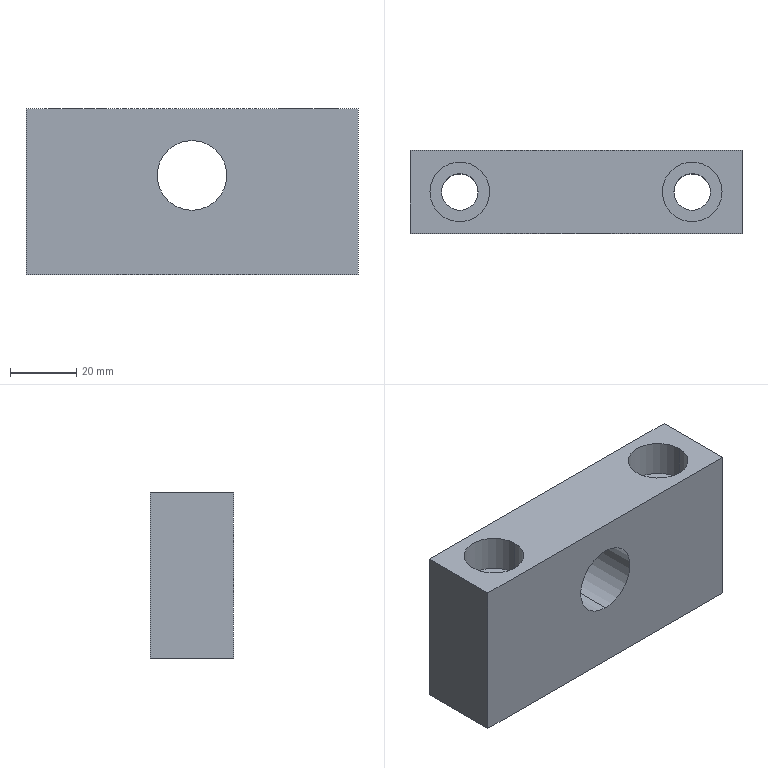Part | SolidWorks | features BaseBody 1 | 1 solid | 26 faces | box 100 x 25 x 50 mm | volume 100070 mm3 | cylinder 14 | plane 8 | cone 4 | commonest cylinder face diameters 10 x4 11 x4 18 x4 21 x2
STEP:
#1=CARTESIAN_POINT('',(20.,0.,19.75));
#2=VERTEX_POINT('',#1);
#3=CARTESIAN_POINT('',(10.,0.,19.75));
#4=VERTEX_POINT('',#3);
#5=CARTESIAN_POINT('',(15.,0.,19.75));
#6=DIRECTION('',(0.,0.,-1.));
#7=DIRECTION('',(-1.,0.,0.));
#8=AXIS2_PLACEMENT_3D('',#5,#6,#7);
#9=CIRCLE('',#8,5.);
#10=EDGE_CURVE('',#2,#4,#9,.T.);
#11=ORIENTED_EDGE('',*,*,#10,.F.);
#12=CARTESIAN_POINT('',(20.,0.,0.));
#13=VERTEX_POINT('',#12);
#14=CARTESIAN_POINT('',(20.,0.,0.));
#15=DIRECTION('',(0.,0.,-1.));
#16=VECTOR('',#15,1000.);
#17=LINE('',#14,#16);
#18=EDGE_CURVE('',#2,#13,#17,.T.);
#19=ORIENTED_EDGE('',*,*,#18,.T.);
#20=CARTESIAN_POINT('',(10.,0.,0.));
#21=VERTEX_POINT('',#20);
#22=CARTESIAN_POINT('',(15.,0.,0.));
#23=DIRECTION('',(0.,0.,-1.));
#24=DIRECTION('',(-1.,0.,0.));
#25=AXIS2_PLACEMENT_3D('',#22,#23,#24);
#26=CIRCLE('',#25,5.);
#27=EDGE_CURVE('',#13,#21,#26,.T.);
#28=ORIENTED_EDGE('',*,*,#27,.T.);
#29=CARTESIAN_POINT('',(10.,0.,0.));
#30=DIRECTION('',(0.,0.,-1.));
#31=VECTOR('',#30,1000.);
#32=LINE('',#29,#31);
#33=EDGE_CURVE('',#4,#21,#32,.T.);
#34=ORIENTED_EDGE('',*,*,#33,.F.);
#35=EDGE_LOOP('',(#11,#19,#28,#34));
#36=FACE_OUTER_BOUND('',#35,.T.);
#37=CARTESIAN_POINT('',(15.,0.,0.));
#38=DIRECTION('',(0.,0.,-1.));
#39=DIRECTION('',(-1.,0.,0.));
#40=AXIS2_PLACEMENT_3D('',#37,#38,#39);
#41=CYLINDRICAL_SURFACE('',#40,5.);
#42=ADVANCED_FACE('',(#36),#41,.F.);
#43=CARTESIAN_POINT('',(15.,0.,22.754));
#44=VERTEX_POINT('',#43);
#45=CARTESIAN_POINT('',(10.,0.,19.75));
#46=DIRECTION('',(-0.8572,0.,-0.515));
#47=VECTOR('',#46,1000.);
#48=LINE('',#45,#47);
#49=EDGE_CURVE('',#44,#4,#48,.T.);
#50=ORIENTED_EDGE('',*,*,#49,.F.);
#51=CARTESIAN_POINT('',(20.,0.,19.75));
#52=DIRECTION('',(0.8572,0.,-0.515));
#53=VECTOR('',#52,1000.);
#54=LINE('',#51,#53);
#55=EDGE_CURVE('',#44,#2,#54,.T.);
#56=ORIENTED_EDGE('',*,*,#55,.T.);
#57=ORIENTED_EDGE('',*,*,#10,.T.);
#58=EDGE_LOOP('',(#50,#56,#57));
#59=FACE_OUTER_BOUND('',#58,.T.);
#60=CARTESIAN_POINT('',(15.,0.,19.75));
#61=DIRECTION('',(0.,0.,-1.));
#62=DIRECTION('',(-1.,0.,0.));
#63=AXIS2_PLACEMENT_3D('',#60,#61,#62);
#64=CONICAL_SURFACE('',#63,5.,1.03);
#65=ADVANCED_FACE('',(#59),#64,.F.);
#66=CARTESIAN_POINT('',(-10.,0.,19.75));
#67=VERTEX_POINT('',#66);
#68=CARTESIAN_POINT('',(-20.,0.,19.75));
#69=VERTEX_POINT('',#68);
#70=CARTESIAN_POINT('',(-15.,0.,19.75));
#71=DIRECTION('',(0.,0.,-1.));
#72=DIRECTION('',(-1.,0.,0.));
#73=AXIS2_PLACEMENT_3D('',#70,#71,#72);
#74=CIRCLE('',#73,5.);
#75=EDGE_CURVE('',#67,#69,#74,.T.);
#76=ORIENTED_EDGE('',*,*,#75,.F.);
#77=CARTESIAN_POINT('',(-10.,0.,0.));
#78=VERTEX_POINT('',#77);
#79=CARTESIAN_POINT('',(-10.,0.,0.));
#80=DIRECTION('',(0.,0.,-1.));
#81=VECTOR('',#80,1000.);
#82=LINE('',#79,#81);
#83=EDGE_CURVE('',#67,#78,#82,.T.);
#84=ORIENTED_EDGE('',*,*,#83,.T.);
#85=CARTESIAN_POINT('',(-20.,0.,0.));
#86=VERTEX_POINT('',#85);
#87=CARTESIAN_POINT('',(-15.,0.,0.));
#88=DIRECTION('',(0.,0.,-1.));
#89=DIRECTION('',(-1.,0.,0.));
#90=AXIS2_PLACEMENT_3D('',#87,#88,#89);
#91=CIRCLE('',#90,5.);
#92=EDGE_CURVE('',#78,#86,#91,.T.);
#93=ORIENTED_EDGE('',*,*,#92,.T.);
#94=CARTESIAN_POINT('',(-20.,0.,0.));
#95=DIRECTION('',(0.,0.,-1.));
#96=VECTOR('',#95,1000.);
#97=LINE('',#94,#96);
#98=EDGE_CURVE('',#69,#86,#97,.T.);
#99=ORIENTED_EDGE('',*,*,#98,.F.);
#100=EDGE_LOOP('',(#76,#84,#93,#99));
#101=FACE_OUTER_BOUND('',#100,.T.);
#102=CARTESIAN_POINT('',(-15.,0.,0.));
#103=DIRECTION('',(0.,0.,-1.));
#104=DIRECTION('',(-1.,0.,0.));
#105=AXIS2_PLACEMENT_3D('',#102,#103,#104);
#106=CYLINDRICAL_SURFACE('',#105,5.);
#107=ADVANCED_FACE('',(#101),#106,.F.);
#108=CARTESIAN_POINT('',(-15.,0.,22.754));
#109=VERTEX_POINT('',#108);
#110=CARTESIAN_POINT('',(-20.,0.,19.75));
#111=DIRECTION('',(-0.8572,0.,-0.515));
#112=VECTOR('',#111,1000.);
#113=LINE('',#110,#112);
#114=EDGE_CURVE('',#109,#69,#113,.T.);
#115=ORIENTED_EDGE('',*,*,#114,.F.);
#116=CARTESIAN_POINT('',(-10.,0.,19.75));
#117=DIRECTION('',(0.8572,0.,-0.515));
#118=VECTOR('',#117,1000.);
#119=LINE('',#116,#118);
#120=EDGE_CURVE('',#109,#67,#119,.T.);
#121=ORIENTED_EDGE('',*,*,#120,.T.);
#122=ORIENTED_EDGE('',*,*,#75,.T.);
#123=EDGE_LOOP('',(#115,#121,#122));
#124=FACE_OUTER_BOUND('',#123,.T.);
#125=CARTESIAN_POINT('',(-15.,0.,19.75));
#126=DIRECTION('',(0.,0.,-1.));
#127=DIRECTION('',(-1.,0.,0.));
#128=AXIS2_PLACEMENT_3D('',#125,#126,#127);
#129=CONICAL_SURFACE('',#128,5.,1.03);
#130=ADVANCED_FACE('',(#124),#129,.F.);
#131=CARTESIAN_POINT('',(0.,-12.5,19.5));
#132=VERTEX_POINT('',#131);
#133=CARTESIAN_POINT('',(0.,-12.5,40.5));
#134=VERTEX_POINT('',#133);
#135=CARTESIAN_POINT('',(0.,-12.5,30.));
#136=DIRECTION('',(0.,1.,0.));
#137=DIRECTION('',(0.,0.,1.));
#138=AXIS2_PLACEMENT_3D('',#135,#136,#137);
#139=CIRCLE('',#138,10.5);
#140=EDGE_CURVE('',#132,#134,#139,.T.);
#141=ORIENTED_EDGE('',*,*,#140,.F.);
#142=CARTESIAN_POINT('',(0.,12.5,19.5));
#143=VERTEX_POINT('',#142);
#144=CARTESIAN_POINT('',(0.,12.5,19.5));
#145=DIRECTION('',(0.,1.,0.));
#146=VECTOR('',#145,1000.);
#147=LINE('',#144,#146);
#148=EDGE_CURVE('',#132,#143,#147,.T.);
#149=ORIENTED_EDGE('',*,*,#148,.T.);
#150=CARTESIAN_POINT('',(0.,12.5,40.5));
#151=VERTEX_POINT('',#150);
#152=CARTESIAN_POINT('',(0.,12.5,30.));
#153=DIRECTION('',(0.,1.,0.));
#154=DIRECTION('',(0.,0.,1.));
#155=AXIS2_PLACEMENT_3D('',#152,#153,#154);
#156=CIRCLE('',#155,10.5);
#157=EDGE_CURVE('',#143,#151,#156,.T.);
#158=ORIENTED_EDGE('',*,*,#157,.T.);
#159=CARTESIAN_POINT('',(0.,12.5,40.5));
#160=DIRECTION('',(0.,1.,0.));
#161=VECTOR('',#160,1000.);
#162=LINE('',#159,#161);
#163=EDGE_CURVE('',#134,#151,#162,.T.);
#164=ORIENTED_EDGE('',*,*,#163,.F.);
#165=EDGE_LOOP('',(#141,#149,#158,#164));
#166=FACE_OUTER_BOUND('',#165,.T.);
#167=CARTESIAN_POINT('',(0.,12.5,30.));
#168=DIRECTION('',(0.,1.,0.));
#169=DIRECTION('',(0.,0.,1.));
#170=AXIS2_PLACEMENT_3D('',#167,#168,#169);
#171=CYLINDRICAL_SURFACE('',#170,10.5);
#172=ADVANCED_FACE('',(#166),#171,.F.);
#173=CARTESIAN_POINT('',(-44.,0.,39.));
#174=VERTEX_POINT('',#173);
#175=CARTESIAN_POINT('',(-26.,0.,39.));
#176=VERTEX_POINT('',#175);
#177=CARTESIAN_POINT('',(-35.,0.,39.));
#178=DIRECTION('',(0.,0.,1.));
#179=DIRECTION('',(1.,0.,0.));
#180=AXIS2_PLACEMENT_3D('',#177,#178,#179);
#181=CIRCLE('',#180,9.);
#182=EDGE_CURVE('',#174,#176,#181,.T.);
#183=ORIENTED_EDGE('',*,*,#182,.F.);
#184=CARTESIAN_POINT('',(-44.,0.,50.));
#185=VERTEX_POINT('',#184);
#186=CARTESIAN_POINT('',(-44.,0.,50.));
#187=DIRECTION('',(0.,0.,1.));
#188=VECTOR('',#187,1000.);
#189=LINE('',#186,#188);
#190=EDGE_CURVE('',#174,#185,#189,.T.);
#191=ORIENTED_EDGE('',*,*,#190,.T.);
#192=CARTESIAN_POINT('',(-26.,0.,50.));
#193=VERTEX_POINT('',#192);
#194=CARTESIAN_POINT('',(-35.,0.,50.));
#195=DIRECTION('',(0.,0.,1.));
#196=DIRECTION('',(1.,0.,0.));
#197=AXIS2_PLACEMENT_3D('',#194,#195,#196);
#198=CIRCLE('',#197,9.);
#199=EDGE_CURVE('',#185,#193,#198,.T.);
#200=ORIENTED_EDGE('',*,*,#199,.T.);
#201=CARTESIAN_POINT('',(-26.,0.,50.));
#202=DIRECTION('',(0.,0.,1.));
#203=VECTOR('',#202,1000.);
#204=LINE('',#201,#203);
#205=EDGE_CURVE('',#176,#193,#204,.T.);
#206=ORIENTED_EDGE('',*,*,#205,.F.);
#207=EDGE_LOOP('',(#183,#191,#200,#206));
#208=FACE_OUTER_BOUND('',#207,.T.);
#209=CARTESIAN_POINT('',(-35.,0.,50.));
#210=DIRECTION('',(0.,0.,1.));
#211=DIRECTION('',(1.,0.,0.));
#212=AXIS2_PLACEMENT_3D('',#209,#210,#211);
#213=CYLINDRICAL_SURFACE('',#212,9.);
#214=ADVANCED_FACE('',(#208),#213,.F.);
#215=CARTESIAN_POINT('',(-40.5,0.,0.));
#216=VERTEX_POINT('',#215);
#217=CARTESIAN_POINT('',(-29.5,0.,0.));
#218=VERTEX_POINT('',#217);
#219=CARTESIAN_POINT('',(-35.,0.,0.));
#220=DIRECTION('',(0.,0.,1.));
#221=DIRECTION('',(1.,0.,0.));
#222=AXIS2_PLACEMENT_3D('',#219,#220,#221);
#223=CIRCLE('',#222,5.5);
#224=EDGE_CURVE('',#216,#218,#223,.T.);
#225=ORIENTED_EDGE('',*,*,#224,.F.);
#226=CARTESIAN_POINT('',(-40.5,0.,39.));
#227=VERTEX_POINT('',#226);
#228=CARTESIAN_POINT('',(-40.5,0.,50.));
#229=DIRECTION('',(0.,0.,1.));
#230=VECTOR('',#229,1000.);
#231=LINE('',#228,#230);
#232=EDGE_CURVE('',#216,#227,#231,.T.);
#233=ORIENTED_EDGE('',*,*,#232,.T.);
#234=CARTESIAN_POINT('',(-29.5,0.,39.));
#235=VERTEX_POINT('',#234);
#236=CARTESIAN_POINT('',(-35.,0.,39.));
#237=DIRECTION('',(0.,0.,1.));
#238=DIRECTION('',(1.,0.,0.));
#239=AXIS2_PLACEMENT_3D('',#236,#237,#238);
#240=CIRCLE('',#239,5.5);
#241=EDGE_CURVE('',#227,#235,#240,.T.);
#242=ORIENTED_EDGE('',*,*,#241,.T.);
#243=CARTESIAN_POINT('',(-29.5,0.,50.));
#244=DIRECTION('',(0.,0.,1.));
#245=VECTOR('',#244,1000.);
#246=LINE('',#243,#245);
#247=EDGE_CURVE('',#218,#235,#246,.T.);
#248=ORIENTED_EDGE('',*,*,#247,.F.);
#249=EDGE_LOOP('',(#225,#233,#242,#248));
#250=FACE_OUTER_BOUND('',#249,.T.);
#251=CARTESIAN_POINT('',(-35.,0.,50.));
#252=DIRECTION('',(0.,0.,1.));
#253=DIRECTION('',(1.,0.,0.));
#254=AXIS2_PLACEMENT_3D('',#251,#252,#253);
#255=CYLINDRICAL_SURFACE('',#254,5.5);
#256=ADVANCED_FACE('',(#250),#255,.F.);
#257=CARTESIAN_POINT('',(26.,0.,39.));
#258=VERTEX_POINT('',#257);
#259=CARTESIAN_POINT('',(44.,0.,39.));
#260=VERTEX_POINT('',#259);
#261=CARTESIAN_POINT('',(35.,0.,39.));
#262=DIRECTION('',(0.,0.,1.));
#263=DIRECTION('',(1.,0.,0.));
#264=AXIS2_PLACEMENT_3D('',#261,#262,#263);
#265=CIRCLE('',#264,9.);
#266=EDGE_CURVE('',#258,#260,#265,.T.);
#267=ORIENTED_EDGE('',*,*,#266,.F.);
#268=CARTESIAN_POINT('',(26.,0.,50.));
#269=VERTEX_POINT('',#268);
#270=CARTESIAN_POINT('',(26.,0.,50.));
#271=DIRECTION('',(0.,0.,1.));
#272=VECTOR('',#271,1000.);
#273=LINE('',#270,#272);
#274=EDGE_CURVE('',#258,#269,#273,.T.);
#275=ORIENTED_EDGE('',*,*,#274,.T.);
#276=CARTESIAN_POINT('',(44.,0.,50.));
#277=VERTEX_POINT('',#276);
#278=CARTESIAN_POINT('',(35.,0.,50.));
#279=DIRECTION('',(0.,0.,1.));
#280=DIRECTION('',(1.,0.,0.));
#281=AXIS2_PLACEMENT_3D('',#278,#279,#280);
#282=CIRCLE('',#281,9.);
#283=EDGE_CURVE('',#269,#277,#282,.T.);
#284=ORIENTED_EDGE('',*,*,#283,.T.);
#285=CARTESIAN_POINT('',(44.,0.,50.));
#286=DIRECTION('',(0.,0.,1.));
#287=VECTOR('',#286,1000.);
#288=LINE('',#285,#287);
#289=EDGE_CURVE('',#260,#277,#288,.T.);
#290=ORIENTED_EDGE('',*,*,#289,.F.);
#291=EDGE_LOOP('',(#267,#275,#284,#290));
#292=FACE_OUTER_BOUND('',#291,.T.);
#293=CARTESIAN_POINT('',(35.,0.,50.));
#294=DIRECTION('',(0.,0.,1.));
#295=DIRECTION('',(1.,0.,0.));
#296=AXIS2_PLACEMENT_3D('',#293,#294,#295);
#297=CYLINDRICAL_SURFACE('',#296,9.);
#298=ADVANCED_FACE('',(#292),#297,.F.);
#299=CARTESIAN_POINT('',(29.5,0.,0.));
#300=VERTEX_POINT('',#299);
#301=CARTESIAN_POINT('',(40.5,0.,0.));
#302=VERTEX_POINT('',#301);
#303=CARTESIAN_POINT('',(35.,0.,0.));
#304=DIRECTION('',(0.,0.,1.));
#305=DIRECTION('',(1.,0.,0.));
#306=AXIS2_PLACEMENT_3D('',#303,#304,#305);
#307=CIRCLE('',#306,5.5);
#308=EDGE_CURVE('',#300,#302,#307,.T.);
#309=ORIENTED_EDGE('',*,*,#308,.F.);
#310=CARTESIAN_POINT('',(29.5,0.,39.));
#311=VERTEX_POINT('',#310);
#312=CARTESIAN_POINT('',(29.5,0.,50.));
#313=DIRECTION('',(0.,0.,1.));
#314=VECTOR('',#313,1000.);
#315=LINE('',#312,#314);
#316=EDGE_CURVE('',#300,#311,#315,.T.);
#317=ORIENTED_EDGE('',*,*,#316,.T.);
#318=CARTESIAN_POINT('',(40.5,0.,39.));
#319=VERTEX_POINT('',#318);
#320=CARTESIAN_POINT('',(35.,0.,39.));
#321=DIRECTION('',(0.,0.,1.));
#322=DIRECTION('',(1.,0.,0.));
#323=AXIS2_PLACEMENT_3D('',#320,#321,#322);
#324=CIRCLE('',#323,5.5);
#325=EDGE_CURVE('',#311,#319,#324,.T.);
#326=ORIENTED_EDGE('',*,*,#325,.T.);
#327=CARTESIAN_POINT('',(40.5,0.,50.));
#328=DIRECTION('',(0.,0.,1.));
#329=VECTOR('',#328,1000.);
#330=LINE('',#327,#329);
#331=EDGE_CURVE('',#302,#319,#330,.T.);
#332=ORIENTED_EDGE('',*,*,#331,.F.);
#333=EDGE_LOOP('',(#309,#317,#326,#332));
#334=FACE_OUTER_BOUND('',#333,.T.);
#335=CARTESIAN_POINT('',(35.,0.,50.));
#336=DIRECTION('',(0.,0.,1.));
#337=DIRECTION('',(1.,0.,0.));
#338=AXIS2_PLACEMENT_3D('',#335,#336,#337);
#339=CYLINDRICAL_SURFACE('',#338,5.5);
#340=ADVANCED_FACE('',(#334),#339,.F.);
#341=CARTESIAN_POINT('',(50.,-12.5,0.));
#342=VERTEX_POINT('',#341);
#343=CARTESIAN_POINT('',(50.,12.5,0.));
#344=VERTEX_POINT('',#343);
#345=CARTESIAN_POINT('',(50.,12.5,0.));
#346=DIRECTION('',(0.,1.,0.));
#347=VECTOR('',#346,1000.);
#348=LINE('',#345,#347);
#349=EDGE_CURVE('',#342,#344,#348,.T.);
#350=ORIENTED_EDGE('',*,*,#349,.T.);
#351=CARTESIAN_POINT('',(50.,12.5,50.));
#352=VERTEX_POINT('',#351);
#353=CARTESIAN_POINT('',(50.,12.5,50.));
#354=DIRECTION('',(0.,0.,-1.));
#355=VECTOR('',#354,1000.);
#356=LINE('',#353,#355);
#357=EDGE_CURVE('',#352,#344,#356,.T.);
#358=ORIENTED_EDGE('',*,*,#357,.F.);
#359=CARTESIAN_POINT('',(50.,-12.5,50.));
#360=VERTEX_POINT('',#359);
#361=CARTESIAN_POINT('',(50.,12.5,50.));
#362=DIRECTION('',(0.,1.,0.));
#363=VECTOR('',#362,1000.);
#364=LINE('',#361,#363);
#365=EDGE_CURVE('',#360,#352,#364,.T.);
#366=ORIENTED_EDGE('',*,*,#365,.F.);
#367=CARTESIAN_POINT('',(50.,-12.5,50.));
#368=DIRECTION('',(0.,0.,-1.));
#369=VECTOR('',#368,1000.);
#370=LINE('',#367,#369);
#371=EDGE_CURVE('',#360,#342,#370,.T.);
#372=ORIENTED_EDGE('',*,*,#371,.T.);
#373=EDGE_LOOP('',(#350,#358,#366,#372));
#374=FACE_OUTER_BOUND('',#373,.T.);
#375=CARTESIAN_POINT('',(50.,12.5,50.));
#376=DIRECTION('',(-1.,0.,0.));
#377=DIRECTION('',(0.,0.,1.));
#378=AXIS2_PLACEMENT_3D('',#375,#376,#377);
#379=PLANE('',#378);
#380=ADVANCED_FACE('',(#374),#379,.F.);
#381=CARTESIAN_POINT('',(0.,12.5,30.));
#382=DIRECTION('',(0.,1.,0.));
#383=DIRECTION('',(0.,0.,1.));
#384=AXIS2_PLACEMENT_3D('',#381,#382,#383);
#385=CIRCLE('',#384,10.5);
#386=EDGE_CURVE('',#151,#143,#385,.T.);
#387=ORIENTED_EDGE('',*,*,#386,.F.);
#388=ORIENTED_EDGE('',*,*,#157,.F.);
#389=EDGE_LOOP('',(#387,#388));
#390=FACE_BOUND('',#389,.T.);
#391=CARTESIAN_POINT('',(-50.,12.5,0.));
#392=VERTEX_POINT('',#391);
#393=CARTESIAN_POINT('',(-50.,12.5,0.));
#394=DIRECTION('',(-1.,0.,0.));
#395=VECTOR('',#394,1000.);
#396=LINE('',#393,#395);
#397=EDGE_CURVE('',#344,#392,#396,.T.);
#398=ORIENTED_EDGE('',*,*,#397,.T.);
#399=CARTESIAN_POINT('',(-50.,12.5,50.));
#400=VERTEX_POINT('',#399);
#401=CARTESIAN_POINT('',(-50.,12.5,50.));
#402=DIRECTION('',(0.,0.,-1.));
#403=VECTOR('',#402,1000.);
#404=LINE('',#401,#403);
#405=EDGE_CURVE('',#400,#392,#404,.T.);
#406=ORIENTED_EDGE('',*,*,#405,.F.);
#407=CARTESIAN_POINT('',(-50.,12.5,50.));
#408=DIRECTION('',(-1.,0.,0.));
#409=VECTOR('',#408,1000.);
#410=LINE('',#407,#409);
#411=EDGE_CURVE('',#352,#400,#410,.T.);
#412=ORIENTED_EDGE('',*,*,#411,.F.);
#413=ORIENTED_EDGE('',*,*,#357,.T.);
#414=EDGE_LOOP('',(#398,#406,#412,#413));
#415=FACE_OUTER_BOUND('',#414,.T.);
#416=CARTESIAN_POINT('',(-50.,12.5,50.));
#417=DIRECTION('',(0.,-1.,0.));
#418=DIRECTION('',(0.,0.,-1.));
#419=AXIS2_PLACEMENT_3D('',#416,#417,#418);
#420=PLANE('',#419);
#421=ADVANCED_FACE('',(#390,#415),#420,.F.);
#422=CARTESIAN_POINT('',(-50.,-12.5,0.));
#423=VERTEX_POINT('',#422);
#424=CARTESIAN_POINT('',(-50.,12.5,0.));
#425=DIRECTION('',(0.,-1.,0.));
#426=VECTOR('',#425,1000.);
#427=LINE('',#424,#426);
#428=EDGE_CURVE('',#392,#423,#427,.T.);
#429=ORIENTED_EDGE('',*,*,#428,.T.);
#430=CARTESIAN_POINT('',(-50.,-12.5,50.));
#431=VERTEX_POINT('',#430);
#432=CARTESIAN_POINT('',(-50.,-12.5,50.));
#433=DIRECTION('',(0.,0.,-1.));
#434=VECTOR('',#433,1000.);
#435=LINE('',#432,#434);
#436=EDGE_CURVE('',#431,#423,#435,.T.);
#437=ORIENTED_EDGE('',*,*,#436,.F.);
#438=CARTESIAN_POINT('',(-50.,12.5,50.));
#439=DIRECTION('',(0.,-1.,0.));
#440=VECTOR('',#439,1000.);
#441=LINE('',#438,#440);
#442=EDGE_CURVE('',#400,#431,#441,.T.);
#443=ORIENTED_EDGE('',*,*,#442,.F.);
#444=ORIENTED_EDGE('',*,*,#405,.T.);
#445=EDGE_LOOP('',(#429,#437,#443,#444));
#446=FACE_OUTER_BOUND('',#445,.T.);
#447=CARTESIAN_POINT('',(-50.,12.5,50.));
#448=DIRECTION('',(1.,0.,0.));
#449=DIRECTION('',(0.,0.,-1.));
#450=AXIS2_PLACEMENT_3D('',#447,#448,#449);
#451=PLANE('',#450);
#452=ADVANCED_FACE('',(#446),#451,.F.);
#453=CARTESIAN_POINT('',(0.,-12.5,30.));
#454=DIRECTION('',(0.,1.,0.));
#455=DIRECTION('',(0.,0.,1.));
#456=AXIS2_PLACEMENT_3D('',#453,#454,#455);
#457=CIRCLE('',#456,10.5);
#458=EDGE_CURVE('',#134,#132,#457,.T.);
#459=ORIENTED_EDGE('',*,*,#458,.T.);
#460=ORIENTED_EDGE('',*,*,#140,.T.);
#461=EDGE_LOOP('',(#459,#460));
#462=FACE_BOUND('',#461,.T.);
#463=CARTESIAN_POINT('',(-50.,-12.5,0.));
#464=DIRECTION('',(1.,0.,0.));
#465=VECTOR('',#464,1000.);
#466=LINE('',#463,#465);
#467=EDGE_CURVE('',#423,#342,#466,.T.);
#468=ORIENTED_EDGE('',*,*,#467,.T.);
#469=ORIENTED_EDGE('',*,*,#371,.F.);
#470=CARTESIAN_POINT('',(-50.,-12.5,50.));
#471=DIRECTION('',(1.,0.,0.));
#472=VECTOR('',#471,1000.);
#473=LINE('',#470,#472);
#474=EDGE_CURVE('',#431,#360,#473,.T.);
#475=ORIENTED_EDGE('',*,*,#474,.F.);
#476=ORIENTED_EDGE('',*,*,#436,.T.);
#477=EDGE_LOOP('',(#468,#469,#475,#476));
#478=FACE_OUTER_BOUND('',#477,.T.);
#479=CARTESIAN_POINT('',(-50.,-12.5,50.));
#480=DIRECTION('',(0.,1.,0.));
#481=DIRECTION('',(0.,0.,1.));
#482=AXIS2_PLACEMENT_3D('',#479,#480,#481);
#483=PLANE('',#482);
#484=ADVANCED_FACE('',(#462,#478),#483,.F.);
#485=CARTESIAN_POINT('',(-35.,0.,50.));
#486=DIRECTION('',(0.,0.,1.));
#487=DIRECTION('',(1.,0.,0.));
#488=AXIS2_PLACEMENT_3D('',#485,#486,#487);
#489=CIRCLE('',#488,9.);
#490=EDGE_CURVE('',#193,#185,#489,.T.);
#491=ORIENTED_EDGE('',*,*,#490,.F.);
#492=ORIENTED_EDGE('',*,*,#199,.F.);
#493=EDGE_LOOP('',(#491,#492));
#494=FACE_BOUND('',#493,.T.);
#495=CARTESIAN_POINT('',(35.,0.,50.));
#496=DIRECTION('',(0.,0.,1.));
#497=DIRECTION('',(1.,0.,0.));
#498=AXIS2_PLACEMENT_3D('',#495,#496,#497);
#499=CIRCLE('',#498,9.);
#500=EDGE_CURVE('',#277,#269,#499,.T.);
#501=ORIENTED_EDGE('',*,*,#500,.F.);
#502=ORIENTED_EDGE('',*,*,#283,.F.);
#503=EDGE_LOOP('',(#501,#502));
#504=FACE_BOUND('',#503,.T.);
#505=ORIENTED_EDGE('',*,*,#365,.T.);
#506=ORIENTED_EDGE('',*,*,#411,.T.);
#507=ORIENTED_EDGE('',*,*,#442,.T.);
#508=ORIENTED_EDGE('',*,*,#474,.T.);
#509=EDGE_LOOP('',(#505,#506,#507,#508));
#510=FACE_OUTER_BOUND('',#509,.T.);
#511=CARTESIAN_POINT('',(0.,0.,50.));
#512=DIRECTION('',(0.,0.,1.));
#513=DIRECTION('',(1.,0.,0.));
#514=AXIS2_PLACEMENT_3D('',#511,#512,#513);
#515=PLANE('',#514);
#516=ADVANCED_FACE('',(#494,#504,#510),#515,.T.);
#517=CARTESIAN_POINT('',(15.,0.,0.));
#518=DIRECTION('',(0.,0.,-1.));
#519=DIRECTION('',(-1.,0.,0.));
#520=AXIS2_PLACEMENT_3D('',#517,#518,#519);
#521=CIRCLE('',#520,5.);
#522=EDGE_CURVE('',#21,#13,#521,.T.);
#523=ORIENTED_EDGE('',*,*,#522,.F.);
#524=ORIENTED_EDGE('',*,*,#27,.F.);
#525=EDGE_LOOP('',(#523,#524));
#526=FACE_BOUND('',#525,.T.);
#527=CARTESIAN_POINT('',(-15.,0.,0.));
#528=DIRECTION('',(0.,0.,-1.));
#529=DIRECTION('',(-1.,0.,0.));
#530=AXIS2_PLACEMENT_3D('',#527,#528,#529);
#531=CIRCLE('',#530,5.);
#532=EDGE_CURVE('',#86,#78,#531,.T.);
#533=ORIENTED_EDGE('',*,*,#532,.F.);
#534=ORIENTED_EDGE('',*,*,#92,.F.);
#535=EDGE_LOOP('',(#533,#534));
#536=FACE_BOUND('',#535,.T.);
#537=CARTESIAN_POINT('',(-35.,0.,0.));
#538=DIRECTION('',(0.,0.,1.));
#539=DIRECTION('',(1.,0.,0.));
#540=AXIS2_PLACEMENT_3D('',#537,#538,#539);
#541=CIRCLE('',#540,5.5);
#542=EDGE_CURVE('',#218,#216,#541,.T.);
#543=ORIENTED_EDGE('',*,*,#542,.T.);
#544=ORIENTED_EDGE('',*,*,#224,.T.);
#545=EDGE_LOOP('',(#543,#544));
#546=FACE_BOUND('',#545,.T.);
#547=CARTESIAN_POINT('',(35.,0.,0.));
#548=DIRECTION('',(0.,0.,1.));
#549=DIRECTION('',(1.,0.,0.));
#550=AXIS2_PLACEMENT_3D('',#547,#548,#549);
#551=CIRCLE('',#550,5.5);
#552=EDGE_CURVE('',#302,#300,#551,.T.);
#553=ORIENTED_EDGE('',*,*,#552,.T.);
#554=ORIENTED_EDGE('',*,*,#308,.T.);
#555=EDGE_LOOP('',(#553,#554));
#556=FACE_BOUND('',#555,.T.);
#557=ORIENTED_EDGE('',*,*,#349,.F.);
#558=ORIENTED_EDGE('',*,*,#467,.F.);
#559=ORIENTED_EDGE('',*,*,#428,.F.);
#560=ORIENTED_EDGE('',*,*,#397,.F.);
#561=EDGE_LOOP('',(#557,#558,#559,#560));
#562=FACE_OUTER_BOUND('',#561,.T.);
#563=CARTESIAN_POINT('',(0.,0.,0.));
#564=DIRECTION('',(0.,0.,1.));
#565=DIRECTION('',(1.,0.,0.));
#566=AXIS2_PLACEMENT_3D('',#563,#564,#565);
#567=PLANE('',#566);
#568=ADVANCED_FACE('',(#526,#536,#546,#556,#562),#567,.F.);
#569=ORIENTED_EDGE('',*,*,#316,.F.);
#570=ORIENTED_EDGE('',*,*,#552,.F.);
#571=ORIENTED_EDGE('',*,*,#331,.T.);
#572=CARTESIAN_POINT('',(35.,0.,39.));
#573=DIRECTION('',(0.,0.,1.));
#574=DIRECTION('',(1.,0.,0.));
#575=AXIS2_PLACEMENT_3D('',#572,#573,#574);
#576=CIRCLE('',#575,5.5);
#577=EDGE_CURVE('',#319,#311,#576,.T.);
#578=ORIENTED_EDGE('',*,*,#577,.T.);
#579=EDGE_LOOP('',(#569,#570,#571,#578));
#580=FACE_OUTER_BOUND('',#579,.T.);
#581=CARTESIAN_POINT('',(35.,0.,50.));
#582=DIRECTION('',(0.,0.,1.));
#583=DIRECTION('',(1.,0.,0.));
#584=AXIS2_PLACEMENT_3D('',#581,#582,#583);
#585=CYLINDRICAL_SURFACE('',#584,5.5);
#586=ADVANCED_FACE('',(#580),#585,.F.);
#587=ORIENTED_EDGE('',*,*,#577,.F.);
#588=ORIENTED_EDGE('',*,*,#325,.F.);
#589=EDGE_LOOP('',(#587,#588));
#590=FACE_BOUND('',#589,.T.);
#591=CARTESIAN_POINT('',(35.,0.,39.));
#592=DIRECTION('',(0.,0.,1.));
#593=DIRECTION('',(1.,0.,0.));
#594=AXIS2_PLACEMENT_3D('',#591,#592,#593);
#595=CIRCLE('',#594,9.);
#596=EDGE_CURVE('',#260,#258,#595,.T.);
#597=ORIENTED_EDGE('',*,*,#596,.T.);
#598=ORIENTED_EDGE('',*,*,#266,.T.);
#599=EDGE_LOOP('',(#597,#598));
#600=FACE_OUTER_BOUND('',#599,.T.);
#601=CARTESIAN_POINT('',(40.5,0.,39.));
#602=DIRECTION('',(0.,0.,-1.));
#603=DIRECTION('',(-1.,0.,0.));
#604=AXIS2_PLACEMENT_3D('',#601,#602,#603);
#605=PLANE('',#604);
#606=ADVANCED_FACE('',(#590,#600),#605,.F.);
#607=ORIENTED_EDGE('',*,*,#274,.F.);
#608=ORIENTED_EDGE('',*,*,#596,.F.);
#609=ORIENTED_EDGE('',*,*,#289,.T.);
#610=ORIENTED_EDGE('',*,*,#500,.T.);
#611=EDGE_LOOP('',(#607,#608,#609,#610));
#612=FACE_OUTER_BOUND('',#611,.T.);
#613=CARTESIAN_POINT('',(35.,0.,50.));
#614=DIRECTION('',(0.,0.,1.));
#615=DIRECTION('',(1.,0.,0.));
#616=AXIS2_PLACEMENT_3D('',#613,#614,#615);
#617=CYLINDRICAL_SURFACE('',#616,9.);
#618=ADVANCED_FACE('',(#612),#617,.F.);
#619=ORIENTED_EDGE('',*,*,#232,.F.);
#620=ORIENTED_EDGE('',*,*,#542,.F.);
#621=ORIENTED_EDGE('',*,*,#247,.T.);
#622=CARTESIAN_POINT('',(-35.,0.,39.));
#623=DIRECTION('',(0.,0.,1.));
#624=DIRECTION('',(1.,0.,0.));
#625=AXIS2_PLACEMENT_3D('',#622,#623,#624);
#626=CIRCLE('',#625,5.5);
#627=EDGE_CURVE('',#235,#227,#626,.T.);
#628=ORIENTED_EDGE('',*,*,#627,.T.);
#629=EDGE_LOOP('',(#619,#620,#621,#628));
#630=FACE_OUTER_BOUND('',#629,.T.);
#631=CARTESIAN_POINT('',(-35.,0.,50.));
#632=DIRECTION('',(0.,0.,1.));
#633=DIRECTION('',(1.,0.,0.));
#634=AXIS2_PLACEMENT_3D('',#631,#632,#633);
#635=CYLINDRICAL_SURFACE('',#634,5.5);
#636=ADVANCED_FACE('',(#630),#635,.F.);
#637=ORIENTED_EDGE('',*,*,#627,.F.);
#638=ORIENTED_EDGE('',*,*,#241,.F.);
#639=EDGE_LOOP('',(#637,#638));
#640=FACE_BOUND('',#639,.T.);
#641=CARTESIAN_POINT('',(-35.,0.,39.));
#642=DIRECTION('',(0.,0.,1.));
#643=DIRECTION('',(1.,0.,0.));
#644=AXIS2_PLACEMENT_3D('',#641,#642,#643);
#645=CIRCLE('',#644,9.);
#646=EDGE_CURVE('',#176,#174,#645,.T.);
#647=ORIENTED_EDGE('',*,*,#646,.T.);
#648=ORIENTED_EDGE('',*,*,#182,.T.);
#649=EDGE_LOOP('',(#647,#648));
#650=FACE_OUTER_BOUND('',#649,.T.);
#651=CARTESIAN_POINT('',(-29.5,0.,39.));
#652=DIRECTION('',(0.,0.,-1.));
#653=DIRECTION('',(-1.,0.,0.));
#654=AXIS2_PLACEMENT_3D('',#651,#652,#653);
#655=PLANE('',#654);
#656=ADVANCED_FACE('',(#640,#650),#655,.F.);
#657=ORIENTED_EDGE('',*,*,#190,.F.);
#658=ORIENTED_EDGE('',*,*,#646,.F.);
#659=ORIENTED_EDGE('',*,*,#205,.T.);
#660=ORIENTED_EDGE('',*,*,#490,.T.);
#661=EDGE_LOOP('',(#657,#658,#659,#660));
#662=FACE_OUTER_BOUND('',#661,.T.);
#663=CARTESIAN_POINT('',(-35.,0.,50.));
#664=DIRECTION('',(0.,0.,1.));
#665=DIRECTION('',(1.,0.,0.));
#666=AXIS2_PLACEMENT_3D('',#663,#664,#665);
#667=CYLINDRICAL_SURFACE('',#666,9.);
#668=ADVANCED_FACE('',(#662),#667,.F.);
#669=ORIENTED_EDGE('',*,*,#148,.F.);
#670=ORIENTED_EDGE('',*,*,#458,.F.);
#671=ORIENTED_EDGE('',*,*,#163,.T.);
#672=ORIENTED_EDGE('',*,*,#386,.T.);
#673=EDGE_LOOP('',(#669,#670,#671,#672));
#674=FACE_OUTER_BOUND('',#673,.T.);
#675=CARTESIAN_POINT('',(0.,12.5,30.));
#676=DIRECTION('',(0.,1.,0.));
#677=DIRECTION('',(0.,0.,1.));
#678=AXIS2_PLACEMENT_3D('',#675,#676,#677);
#679=CYLINDRICAL_SURFACE('',#678,10.5);
#680=ADVANCED_FACE('',(#674),#679,.F.);
#681=ORIENTED_EDGE('',*,*,#120,.F.);
#682=ORIENTED_EDGE('',*,*,#114,.T.);
#683=CARTESIAN_POINT('',(-15.,0.,19.75));
#684=DIRECTION('',(0.,0.,-1.));
#685=DIRECTION('',(-1.,0.,0.));
#686=AXIS2_PLACEMENT_3D('',#683,#684,#685);
#687=CIRCLE('',#686,5.);
#688=EDGE_CURVE('',#69,#67,#687,.T.);
#689=ORIENTED_EDGE('',*,*,#688,.T.);
#690=EDGE_LOOP('',(#681,#682,#689));
#691=FACE_OUTER_BOUND('',#690,.T.);
#692=CARTESIAN_POINT('',(-15.,0.,19.75));
#693=DIRECTION('',(0.,0.,-1.));
#694=DIRECTION('',(-1.,0.,0.));
#695=AXIS2_PLACEMENT_3D('',#692,#693,#694);
#696=CONICAL_SURFACE('',#695,5.,1.03);
#697=ADVANCED_FACE('',(#691),#696,.F.);
#698=ORIENTED_EDGE('',*,*,#83,.F.);
#699=ORIENTED_EDGE('',*,*,#688,.F.);
#700=ORIENTED_EDGE('',*,*,#98,.T.);
#701=ORIENTED_EDGE('',*,*,#532,.T.);
#702=EDGE_LOOP('',(#698,#699,#700,#701));
#703=FACE_OUTER_BOUND('',#702,.T.);
#704=CARTESIAN_POINT('',(-15.,0.,0.));
#705=DIRECTION('',(0.,0.,-1.));
#706=DIRECTION('',(-1.,0.,0.));
#707=AXIS2_PLACEMENT_3D('',#704,#705,#706);
#708=CYLINDRICAL_SURFACE('',#707,5.);
#709=ADVANCED_FACE('',(#703),#708,.F.);
#710=ORIENTED_EDGE('',*,*,#55,.F.);
#711=ORIENTED_EDGE('',*,*,#49,.T.);
#712=CARTESIAN_POINT('',(15.,0.,19.75));
#713=DIRECTION('',(0.,0.,-1.));
#714=DIRECTION('',(-1.,0.,0.));
#715=AXIS2_PLACEMENT_3D('',#712,#713,#714);
#716=CIRCLE('',#715,5.);
#717=EDGE_CURVE('',#4,#2,#716,.T.);
#718=ORIENTED_EDGE('',*,*,#717,.T.);
#719=EDGE_LOOP('',(#710,#711,#718));
#720=FACE_OUTER_BOUND('',#719,.T.);
#721=CARTESIAN_POINT('',(15.,0.,19.75));
#722=DIRECTION('',(0.,0.,-1.));
#723=DIRECTION('',(-1.,0.,0.));
#724=AXIS2_PLACEMENT_3D('',#721,#722,#723);
#725=CONICAL_SURFACE('',#724,5.,1.03);
#726=ADVANCED_FACE('',(#720),#725,.F.);
#727=ORIENTED_EDGE('',*,*,#18,.F.);
#728=ORIENTED_EDGE('',*,*,#717,.F.);
#729=ORIENTED_EDGE('',*,*,#33,.T.);
#730=ORIENTED_EDGE('',*,*,#522,.T.);
#731=EDGE_LOOP('',(#727,#728,#729,#730));
#732=FACE_OUTER_BOUND('',#731,.T.);
#733=CARTESIAN_POINT('',(15.,0.,0.));
#734=DIRECTION('',(0.,0.,-1.));
#735=DIRECTION('',(-1.,0.,0.));
#736=AXIS2_PLACEMENT_3D('',#733,#734,#735);
#737=CYLINDRICAL_SURFACE('',#736,5.);
#738=ADVANCED_FACE('',(#732),#737,.F.);
#739=CLOSED_SHELL('',(#42,#65,#107,#130,#172,#214,#256,#298,#340,#380,#421,#452,#484,#516,#568,#586,#606,#618,#636,#656,#668,#680,#697,#709,#726,#738));
#740=MANIFOLD_SOLID_BREP('',#739);
#741=CARTESIAN_POINT('',(0.,0.,0.));
#742=DIRECTION('',(0.,0.,1.));
#743=DIRECTION('',(1.,0.,0.));
#744=AXIS2_PLACEMENT_3D('',#741,#742,#743);
#745=(LENGTH_UNIT()NAMED_UNIT(*)SI_UNIT(.MILLI.,.METRE.));
#746=UNCERTAINTY_MEASURE_WITH_UNIT(LENGTH_MEASURE(0.00001),#745,'','');
#747=(NAMED_UNIT(*)PLANE_ANGLE_UNIT()SI_UNIT($,.RADIAN.));
#748=(NAMED_UNIT(*)SI_UNIT($,.STERADIAN.)SOLID_ANGLE_UNIT());
#749=(GEOMETRIC_REPRESENTATION_CONTEXT(3)GLOBAL_UNCERTAINTY_ASSIGNED_CONTEXT((#746))GLOBAL_UNIT_ASSIGNED_CONTEXT((#745,#747,#748))REPRESENTATION_CONTEXT('',''));
#750=ADVANCED_BREP_SHAPE_REPRESENTATION('',(#740,#744),#749);